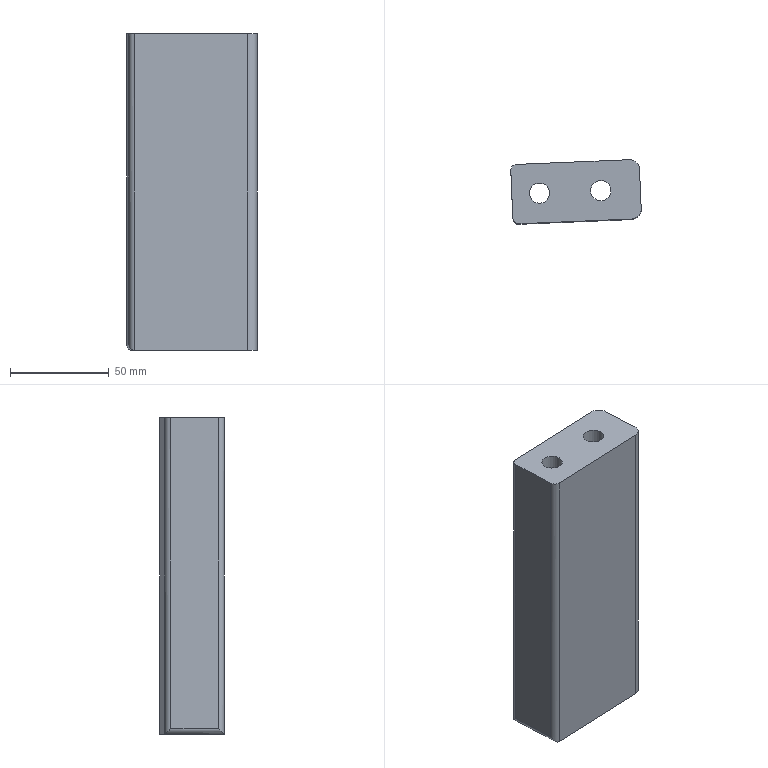Part | NX | features 8 2 | 1 solid | 17 faces | box 65.871 x 32.366 x 160 mm | volume 238451 mm3 | cylinder 9 | plane 8 | commonest cylinder face diameters 6 x3 10 x2 10.3 x2 18 x2
STEP:
#1=CARTESIAN_POINT('',(3750.311,363.335,-69.));
#2=VERTEX_POINT('',#1);
#3=CARTESIAN_POINT('',(3750.311,363.335,91.));
#4=VERTEX_POINT('',#3);
#5=CARTESIAN_POINT('',(3750.311,363.335,-9.));
#6=DIRECTION('',(0.,0.,1.));
#7=VECTOR('',#6,1000.);
#8=LINE('',#5,#7);
#9=EDGE_CURVE('',#2,#4,#8,.T.);
#10=ORIENTED_EDGE('',*,*,#9,.F.);
#11=CARTESIAN_POINT('',(3693.361,360.951,-69.));
#12=VERTEX_POINT('',#11);
#13=CARTESIAN_POINT('',(3740.32,362.917,-69.));
#14=DIRECTION('',(-0.9991,-0.04184,0.));
#15=VECTOR('',#14,1000.);
#16=LINE('',#13,#15);
#17=EDGE_CURVE('',#2,#12,#16,.T.);
#18=ORIENTED_EDGE('',*,*,#17,.T.);
#19=CARTESIAN_POINT('',(3693.361,360.951,91.));
#20=VERTEX_POINT('',#19);
#21=CARTESIAN_POINT('',(3693.361,360.951,-9.));
#22=DIRECTION('',(0.,0.,-1.));
#23=VECTOR('',#22,1000.);
#24=LINE('',#21,#23);
#25=EDGE_CURVE('',#20,#12,#24,.T.);
#26=ORIENTED_EDGE('',*,*,#25,.F.);
#27=CARTESIAN_POINT('',(3740.32,362.917,91.));
#28=DIRECTION('',(-0.9991,-0.04184,0.));
#29=VECTOR('',#28,1000.);
#30=LINE('',#27,#29);
#31=EDGE_CURVE('',#4,#20,#30,.T.);
#32=ORIENTED_EDGE('',*,*,#31,.F.);
#33=EDGE_LOOP('',(#10,#18,#26,#32));
#34=FACE_BOUND('',#33,.T.);
#35=CARTESIAN_POINT('',(3740.32,362.917,-9.));
#36=DIRECTION('',(-0.04184,0.9991,0.));
#37=DIRECTION('',(0.,0.,1.));
#38=AXIS2_PLACEMENT_3D('',#35,#36,#37);
#39=PLANE('',#38);
#40=ADVANCED_FACE('',(#34),#39,.T.);
#41=CARTESIAN_POINT('',(3756.353,338.567,-69.));
#42=VERTEX_POINT('',#41);
#43=CARTESIAN_POINT('',(3756.353,338.567,91.));
#44=VERTEX_POINT('',#43);
#45=CARTESIAN_POINT('',(3756.353,338.567,-9.));
#46=DIRECTION('',(0.,0.,1.));
#47=VECTOR('',#46,1000.);
#48=LINE('',#45,#47);
#49=EDGE_CURVE('',#42,#44,#48,.T.);
#50=ORIENTED_EDGE('',*,*,#49,.F.);
#51=CARTESIAN_POINT('',(3755.516,358.549,-69.));
#52=VERTEX_POINT('',#51);
#53=CARTESIAN_POINT('',(3755.934,348.558,-69.));
#54=DIRECTION('',(-0.04184,0.9991,0.));
#55=VECTOR('',#54,1000.);
#56=LINE('',#53,#55);
#57=EDGE_CURVE('',#42,#52,#56,.T.);
#58=ORIENTED_EDGE('',*,*,#57,.T.);
#59=CARTESIAN_POINT('',(3755.516,358.549,91.));
#60=VERTEX_POINT('',#59);
#61=CARTESIAN_POINT('',(3755.516,358.549,-9.));
#62=DIRECTION('',(0.,0.,-1.));
#63=VECTOR('',#62,1000.);
#64=LINE('',#61,#63);
#65=EDGE_CURVE('',#60,#52,#64,.T.);
#66=ORIENTED_EDGE('',*,*,#65,.F.);
#67=CARTESIAN_POINT('',(3755.934,348.558,91.));
#68=DIRECTION('',(-0.04184,0.9991,0.));
#69=VECTOR('',#68,1000.);
#70=LINE('',#67,#69);
#71=EDGE_CURVE('',#44,#60,#70,.T.);
#72=ORIENTED_EDGE('',*,*,#71,.F.);
#73=EDGE_LOOP('',(#50,#58,#66,#72));
#74=FACE_BOUND('',#73,.T.);
#75=CARTESIAN_POINT('',(3755.934,348.558,-9.));
#76=DIRECTION('',(0.9991,0.04184,0.));
#77=DIRECTION('',(0.,0.,-1.));
#78=AXIS2_PLACEMENT_3D('',#75,#76,#77);
#79=PLANE('',#78);
#80=ADVANCED_FACE('',(#74),#79,.T.);
#81=CARTESIAN_POINT('',(3690.489,357.828,-66.));
#82=VERTEX_POINT('',#81);
#83=CARTESIAN_POINT('',(3690.489,357.828,91.));
#84=VERTEX_POINT('',#83);
#85=CARTESIAN_POINT('',(3690.489,357.828,-9.));
#86=DIRECTION('',(0.,0.,1.));
#87=VECTOR('',#86,1000.);
#88=LINE('',#85,#87);
#89=EDGE_CURVE('',#82,#84,#88,.T.);
#90=ORIENTED_EDGE('',*,*,#89,.F.);
#91=CARTESIAN_POINT('',(3691.493,333.849,-66.));
#92=VERTEX_POINT('',#91);
#93=CARTESIAN_POINT('',(3690.991,345.838,-66.));
#94=DIRECTION('',(0.04184,-0.9991,0.));
#95=VECTOR('',#94,1000.);
#96=LINE('',#93,#95);
#97=EDGE_CURVE('',#82,#92,#96,.T.);
#98=ORIENTED_EDGE('',*,*,#97,.T.);
#99=CARTESIAN_POINT('',(3691.493,333.849,91.));
#100=VERTEX_POINT('',#99);
#101=CARTESIAN_POINT('',(3691.493,333.849,-9.));
#102=DIRECTION('',(0.,0.,-1.));
#103=VECTOR('',#102,1000.);
#104=LINE('',#101,#103);
#105=EDGE_CURVE('',#100,#92,#104,.T.);
#106=ORIENTED_EDGE('',*,*,#105,.F.);
#107=CARTESIAN_POINT('',(3690.991,345.838,91.));
#108=DIRECTION('',(0.04184,-0.9991,0.));
#109=VECTOR('',#108,1000.);
#110=LINE('',#107,#109);
#111=EDGE_CURVE('',#84,#100,#110,.T.);
#112=ORIENTED_EDGE('',*,*,#111,.F.);
#113=EDGE_LOOP('',(#90,#98,#106,#112));
#114=FACE_BOUND('',#113,.T.);
#115=CARTESIAN_POINT('',(3690.991,345.838,-9.));
#116=DIRECTION('',(-0.9991,-0.04184,0.));
#117=DIRECTION('',(0.,0.,1.));
#118=AXIS2_PLACEMENT_3D('',#115,#116,#117);
#119=PLANE('',#118);
#120=ADVANCED_FACE('',(#114),#119,.T.);
#121=ORIENTED_EDGE('',*,*,#25,.T.);
#122=CARTESIAN_POINT('',(3693.487,357.953,-66.));
#123=DIRECTION('',(-0.02958,0.7065,0.7071));
#124=DIRECTION('',(-0.02958,0.7065,-0.7071));
#125=AXIS2_PLACEMENT_3D('',#122,#123,#124);
#126=ELLIPSE('',#125,4.243,3.);
#127=EDGE_CURVE('',#12,#82,#126,.T.);
#128=ORIENTED_EDGE('',*,*,#127,.T.);
#129=ORIENTED_EDGE('',*,*,#89,.T.);
#130=CARTESIAN_POINT('',(3693.487,357.953,91.));
#131=DIRECTION('',(0.,0.,-1.));
#132=DIRECTION('',(1.,0.,0.));
#133=AXIS2_PLACEMENT_3D('',#130,#131,#132);
#134=CIRCLE('',#133,3.);
#135=EDGE_CURVE('',#84,#20,#134,.T.);
#136=ORIENTED_EDGE('',*,*,#135,.T.);
#137=EDGE_LOOP('',(#121,#128,#129,#136));
#138=FACE_BOUND('',#137,.T.);
#139=CARTESIAN_POINT('',(3693.487,357.953,-9.));
#140=DIRECTION('',(0.,0.,-1.));
#141=DIRECTION('',(1.,0.,0.));
#142=AXIS2_PLACEMENT_3D('',#139,#140,#141);
#143=CYLINDRICAL_SURFACE('',#142,3.);
#144=ADVANCED_FACE('',(#138),#143,.T.);
#145=ORIENTED_EDGE('',*,*,#65,.T.);
#146=CARTESIAN_POINT('',(3750.52,358.34,-69.));
#147=DIRECTION('',(0.,0.,1.));
#148=DIRECTION('',(-1.,0.,0.));
#149=AXIS2_PLACEMENT_3D('',#146,#147,#148);
#150=CIRCLE('',#149,5.);
#151=EDGE_CURVE('',#52,#2,#150,.T.);
#152=ORIENTED_EDGE('',*,*,#151,.T.);
#153=ORIENTED_EDGE('',*,*,#9,.T.);
#154=CARTESIAN_POINT('',(3750.52,358.34,91.));
#155=DIRECTION('',(0.,0.,-1.));
#156=DIRECTION('',(-0.9991,-0.04184,0.));
#157=AXIS2_PLACEMENT_3D('',#154,#155,#156);
#158=CIRCLE('',#157,5.);
#159=EDGE_CURVE('',#4,#60,#158,.T.);
#160=ORIENTED_EDGE('',*,*,#159,.T.);
#161=EDGE_LOOP('',(#145,#152,#153,#160));
#162=FACE_BOUND('',#161,.T.);
#163=CARTESIAN_POINT('',(3750.52,358.34,-9.));
#164=DIRECTION('',(0.,0.,1.));
#165=DIRECTION('',(0.9991,0.04184,0.));
#166=AXIS2_PLACEMENT_3D('',#163,#164,#165);
#167=CYLINDRICAL_SURFACE('',#166,5.);
#168=ADVANCED_FACE('',(#162),#167,.T.);
#169=CARTESIAN_POINT('',(3744.952,347.721,61.));
#170=VERTEX_POINT('',#169);
#171=CARTESIAN_POINT('',(3735.952,347.721,61.));
#172=DIRECTION('',(0.,0.,-1.));
#173=DIRECTION('',(1.,0.,0.));
#174=AXIS2_PLACEMENT_3D('',#171,#172,#173);
#175=CIRCLE('',#174,9.);
#176=EDGE_CURVE('',#170,#170,#175,.T.);
#177=ORIENTED_EDGE('',*,*,#176,.F.);
#178=EDGE_LOOP('',(#177));
#179=FACE_BOUND('',#178,.T.);
#180=CARTESIAN_POINT('',(3726.952,347.721,-69.));
#181=VERTEX_POINT('',#180);
#182=CARTESIAN_POINT('',(3735.952,347.721,-69.));
#183=DIRECTION('',(0.,0.,1.));
#184=DIRECTION('',(-1.,0.,0.));
#185=AXIS2_PLACEMENT_3D('',#182,#183,#184);
#186=CIRCLE('',#185,9.);
#187=EDGE_CURVE('',#181,#181,#186,.T.);
#188=ORIENTED_EDGE('',*,*,#187,.F.);
#189=EDGE_LOOP('',(#188));
#190=FACE_BOUND('',#189,.T.);
#191=CARTESIAN_POINT('',(3735.952,347.721,-9.));
#192=DIRECTION('',(0.,0.,1.));
#193=DIRECTION('',(0.9991,0.04184,0.));
#194=AXIS2_PLACEMENT_3D('',#191,#192,#193);
#195=CYLINDRICAL_SURFACE('',#194,9.);
#196=ADVANCED_FACE('',(#179,#190),#195,.F.);
#197=CARTESIAN_POINT('',(3741.102,347.721,91.));
#198=VERTEX_POINT('',#197);
#199=CARTESIAN_POINT('',(3735.952,347.721,91.));
#200=DIRECTION('',(0.,0.,1.));
#201=DIRECTION('',(1.,0.,0.));
#202=AXIS2_PLACEMENT_3D('',#199,#200,#201);
#203=CIRCLE('',#202,5.15);
#204=EDGE_CURVE('',#198,#198,#203,.T.);
#205=ORIENTED_EDGE('',*,*,#204,.F.);
#206=EDGE_LOOP('',(#205));
#207=FACE_BOUND('',#206,.T.);
#208=CARTESIAN_POINT('',(3694.616,330.977,91.));
#209=VERTEX_POINT('',#208);
#210=CARTESIAN_POINT('',(3751.566,333.362,91.));
#211=VERTEX_POINT('',#210);
#212=CARTESIAN_POINT('',(3741.575,332.943,91.));
#213=DIRECTION('',(0.9991,0.04184,0.));
#214=VECTOR('',#213,1000.);
#215=LINE('',#212,#214);
#216=EDGE_CURVE('',#209,#211,#215,.T.);
#217=ORIENTED_EDGE('',*,*,#216,.T.);
#218=CARTESIAN_POINT('',(3751.357,338.357,91.));
#219=DIRECTION('',(0.,0.,-1.));
#220=DIRECTION('',(-0.9991,-0.04184,0.));
#221=AXIS2_PLACEMENT_3D('',#218,#219,#220);
#222=CIRCLE('',#221,5.);
#223=EDGE_CURVE('',#44,#211,#222,.T.);
#224=ORIENTED_EDGE('',*,*,#223,.F.);
#225=ORIENTED_EDGE('',*,*,#71,.T.);
#226=ORIENTED_EDGE('',*,*,#159,.F.);
#227=ORIENTED_EDGE('',*,*,#31,.T.);
#228=ORIENTED_EDGE('',*,*,#135,.F.);
#229=ORIENTED_EDGE('',*,*,#111,.T.);
#230=CARTESIAN_POINT('',(3694.491,333.974,91.));
#231=DIRECTION('',(0.,0.,-1.));
#232=DIRECTION('',(1.,0.,0.));
#233=AXIS2_PLACEMENT_3D('',#230,#231,#232);
#234=CIRCLE('',#233,3.);
#235=EDGE_CURVE('',#209,#100,#234,.T.);
#236=ORIENTED_EDGE('',*,*,#235,.F.);
#237=EDGE_LOOP('',(#217,#224,#225,#226,#227,#228,#229,#236));
#238=FACE_BOUND('',#237,.T.);
#239=CARTESIAN_POINT('',(3710.129,346.424,91.));
#240=VERTEX_POINT('',#239);
#241=CARTESIAN_POINT('',(3704.979,346.424,91.));
#242=DIRECTION('',(0.,0.,1.));
#243=DIRECTION('',(1.,0.,0.));
#244=AXIS2_PLACEMENT_3D('',#241,#242,#243);
#245=CIRCLE('',#244,5.15);
#246=EDGE_CURVE('',#240,#240,#245,.T.);
#247=ORIENTED_EDGE('',*,*,#246,.F.);
#248=EDGE_LOOP('',(#247));
#249=FACE_BOUND('',#248,.T.);
#250=CARTESIAN_POINT('',(3740.948,347.93,91.));
#251=DIRECTION('',(0.,0.,1.));
#252=DIRECTION('',(0.9991,0.04184,0.));
#253=AXIS2_PLACEMENT_3D('',#250,#251,#252);
#254=PLANE('',#253);
#255=ADVANCED_FACE('',(#207,#238,#249),#254,.T.);
#256=CARTESIAN_POINT('',(3694.616,330.977,-69.));
#257=VERTEX_POINT('',#256);
#258=CARTESIAN_POINT('',(3694.616,330.977,-9.));
#259=DIRECTION('',(0.,0.,1.));
#260=VECTOR('',#259,1000.);
#261=LINE('',#258,#260);
#262=EDGE_CURVE('',#257,#209,#261,.T.);
#263=ORIENTED_EDGE('',*,*,#262,.F.);
#264=CARTESIAN_POINT('',(3751.566,333.362,-69.));
#265=VERTEX_POINT('',#264);
#266=CARTESIAN_POINT('',(3741.575,332.943,-69.));
#267=DIRECTION('',(-0.9991,-0.04184,0.));
#268=VECTOR('',#267,1000.);
#269=LINE('',#266,#268);
#270=EDGE_CURVE('',#265,#257,#269,.T.);
#271=ORIENTED_EDGE('',*,*,#270,.F.);
#272=CARTESIAN_POINT('',(3751.566,333.362,-9.));
#273=DIRECTION('',(0.,0.,-1.));
#274=VECTOR('',#273,1000.);
#275=LINE('',#272,#274);
#276=EDGE_CURVE('',#211,#265,#275,.T.);
#277=ORIENTED_EDGE('',*,*,#276,.F.);
#278=ORIENTED_EDGE('',*,*,#216,.F.);
#279=EDGE_LOOP('',(#263,#271,#277,#278));
#280=FACE_BOUND('',#279,.T.);
#281=CARTESIAN_POINT('',(3741.575,332.943,-9.));
#282=DIRECTION('',(0.04184,-0.9991,0.));
#283=DIRECTION('',(0.,0.,-1.));
#284=AXIS2_PLACEMENT_3D('',#281,#282,#283);
#285=PLANE('',#284);
#286=ADVANCED_FACE('',(#280),#285,.T.);
#287=ORIENTED_EDGE('',*,*,#276,.T.);
#288=CARTESIAN_POINT('',(3751.357,338.357,-69.));
#289=DIRECTION('',(0.,0.,-1.));
#290=DIRECTION('',(-1.,0.,0.));
#291=AXIS2_PLACEMENT_3D('',#288,#289,#290);
#292=CIRCLE('',#291,5.);
#293=EDGE_CURVE('',#42,#265,#292,.T.);
#294=ORIENTED_EDGE('',*,*,#293,.F.);
#295=ORIENTED_EDGE('',*,*,#49,.T.);
#296=ORIENTED_EDGE('',*,*,#223,.T.);
#297=EDGE_LOOP('',(#287,#294,#295,#296));
#298=FACE_BOUND('',#297,.T.);
#299=CARTESIAN_POINT('',(3751.357,338.357,-9.));
#300=DIRECTION('',(0.,0.,1.));
#301=DIRECTION('',(0.9991,0.04184,0.));
#302=AXIS2_PLACEMENT_3D('',#299,#300,#301);
#303=CYLINDRICAL_SURFACE('',#302,5.);
#304=ADVANCED_FACE('',(#298),#303,.T.);
#305=ORIENTED_EDGE('',*,*,#105,.T.);
#306=CARTESIAN_POINT('',(3694.491,333.974,-66.));
#307=DIRECTION('',(0.02958,-0.7065,0.7071));
#308=DIRECTION('',(0.02958,-0.7065,-0.7071));
#309=AXIS2_PLACEMENT_3D('',#306,#307,#308);
#310=ELLIPSE('',#309,4.243,3.);
#311=EDGE_CURVE('',#92,#257,#310,.T.);
#312=ORIENTED_EDGE('',*,*,#311,.T.);
#313=ORIENTED_EDGE('',*,*,#262,.T.);
#314=ORIENTED_EDGE('',*,*,#235,.T.);
#315=EDGE_LOOP('',(#305,#312,#313,#314));
#316=FACE_BOUND('',#315,.T.);
#317=CARTESIAN_POINT('',(3694.491,333.974,-9.));
#318=DIRECTION('',(0.,0.,-1.));
#319=DIRECTION('',(1.,0.,0.));
#320=AXIS2_PLACEMENT_3D('',#317,#318,#319);
#321=CYLINDRICAL_SURFACE('',#320,3.);
#322=ADVANCED_FACE('',(#316),#321,.T.);
#323=CARTESIAN_POINT('',(3741.102,347.721,61.));
#324=VERTEX_POINT('',#323);
#325=CARTESIAN_POINT('',(3735.952,347.721,61.));
#326=DIRECTION('',(0.,0.,-1.));
#327=DIRECTION('',(1.,0.,0.));
#328=AXIS2_PLACEMENT_3D('',#325,#326,#327);
#329=CIRCLE('',#328,5.15);
#330=EDGE_CURVE('',#324,#324,#329,.T.);
#331=ORIENTED_EDGE('',*,*,#330,.T.);
#332=EDGE_LOOP('',(#331));
#333=FACE_BOUND('',#332,.T.);
#334=ORIENTED_EDGE('',*,*,#204,.T.);
#335=EDGE_LOOP('',(#334));
#336=FACE_BOUND('',#335,.T.);
#337=CARTESIAN_POINT('',(3735.952,347.721,-9.));
#338=DIRECTION('',(0.,0.,1.));
#339=DIRECTION('',(0.9991,0.04184,0.));
#340=AXIS2_PLACEMENT_3D('',#337,#338,#339);
#341=CYLINDRICAL_SURFACE('',#340,5.15);
#342=ADVANCED_FACE('',(#333,#336),#341,.F.);
#343=ORIENTED_EDGE('',*,*,#330,.F.);
#344=EDGE_LOOP('',(#343));
#345=FACE_BOUND('',#344,.T.);
#346=ORIENTED_EDGE('',*,*,#176,.T.);
#347=EDGE_LOOP('',(#346));
#348=FACE_BOUND('',#347,.T.);
#349=CARTESIAN_POINT('',(3752.499,412.84,61.));
#350=DIRECTION('',(0.,0.,1.));
#351=DIRECTION('',(-1.,0.,0.));
#352=AXIS2_PLACEMENT_3D('',#349,#350,#351);
#353=PLANE('',#352);
#354=ADVANCED_FACE('',(#345,#348),#353,.F.);
#355=CARTESIAN_POINT('',(3710.129,346.424,61.));
#356=VERTEX_POINT('',#355);
#357=CARTESIAN_POINT('',(3704.979,346.424,61.));
#358=DIRECTION('',(0.,0.,-1.));
#359=DIRECTION('',(1.,0.,0.));
#360=AXIS2_PLACEMENT_3D('',#357,#358,#359);
#361=CIRCLE('',#360,5.15);
#362=EDGE_CURVE('',#356,#356,#361,.T.);
#363=ORIENTED_EDGE('',*,*,#362,.T.);
#364=EDGE_LOOP('',(#363));
#365=FACE_BOUND('',#364,.T.);
#366=ORIENTED_EDGE('',*,*,#246,.T.);
#367=EDGE_LOOP('',(#366));
#368=FACE_BOUND('',#367,.T.);
#369=CARTESIAN_POINT('',(3704.979,346.424,-9.));
#370=DIRECTION('',(0.,0.,1.));
#371=DIRECTION('',(0.9991,0.04184,0.));
#372=AXIS2_PLACEMENT_3D('',#369,#370,#371);
#373=CYLINDRICAL_SURFACE('',#372,5.15);
#374=ADVANCED_FACE('',(#365,#368),#373,.F.);
#375=ORIENTED_EDGE('',*,*,#362,.F.);
#376=EDGE_LOOP('',(#375));
#377=FACE_BOUND('',#376,.T.);
#378=CARTESIAN_POINT('',(3713.979,346.424,61.));
#379=VERTEX_POINT('',#378);
#380=CARTESIAN_POINT('',(3704.979,346.424,61.));
#381=DIRECTION('',(0.,0.,-1.));
#382=DIRECTION('',(1.,0.,0.));
#383=AXIS2_PLACEMENT_3D('',#380,#381,#382);
#384=CIRCLE('',#383,9.);
#385=EDGE_CURVE('',#379,#379,#384,.T.);
#386=ORIENTED_EDGE('',*,*,#385,.T.);
#387=EDGE_LOOP('',(#386));
#388=FACE_BOUND('',#387,.T.);
#389=CARTESIAN_POINT('',(3752.499,412.84,61.));
#390=DIRECTION('',(0.,0.,1.));
#391=DIRECTION('',(-1.,0.,0.));
#392=AXIS2_PLACEMENT_3D('',#389,#390,#391);
#393=PLANE('',#392);
#394=ADVANCED_FACE('',(#377,#388),#393,.F.);
#395=ORIENTED_EDGE('',*,*,#385,.F.);
#396=EDGE_LOOP('',(#395));
#397=FACE_BOUND('',#396,.T.);
#398=CARTESIAN_POINT('',(3695.979,346.424,-69.));
#399=VERTEX_POINT('',#398);
#400=CARTESIAN_POINT('',(3704.979,346.424,-69.));
#401=DIRECTION('',(0.,0.,-1.));
#402=DIRECTION('',(-1.,0.,0.));
#403=AXIS2_PLACEMENT_3D('',#400,#401,#402);
#404=CIRCLE('',#403,9.);
#405=EDGE_CURVE('',#399,#399,#404,.T.);
#406=ORIENTED_EDGE('',*,*,#405,.T.);
#407=EDGE_LOOP('',(#406));
#408=FACE_BOUND('',#407,.T.);
#409=CARTESIAN_POINT('',(3704.979,346.424,-9.));
#410=DIRECTION('',(0.,0.,1.));
#411=DIRECTION('',(0.9991,0.04184,0.));
#412=AXIS2_PLACEMENT_3D('',#409,#410,#411);
#413=CYLINDRICAL_SURFACE('',#412,9.);
#414=ADVANCED_FACE('',(#397,#408),#413,.F.);
#415=ORIENTED_EDGE('',*,*,#405,.F.);
#416=EDGE_LOOP('',(#415));
#417=FACE_BOUND('',#416,.T.);
#418=ORIENTED_EDGE('',*,*,#270,.T.);
#419=CARTESIAN_POINT('',(3693.99,345.925,-69.));
#420=DIRECTION('',(-0.04184,0.9991,0.));
#421=VECTOR('',#420,1000.);
#422=LINE('',#419,#421);
#423=EDGE_CURVE('',#257,#12,#422,.T.);
#424=ORIENTED_EDGE('',*,*,#423,.T.);
#425=ORIENTED_EDGE('',*,*,#17,.F.);
#426=ORIENTED_EDGE('',*,*,#151,.F.);
#427=ORIENTED_EDGE('',*,*,#57,.F.);
#428=ORIENTED_EDGE('',*,*,#293,.T.);
#429=EDGE_LOOP('',(#418,#424,#425,#426,#427,#428));
#430=FACE_BOUND('',#429,.T.);
#431=ORIENTED_EDGE('',*,*,#187,.T.);
#432=EDGE_LOOP('',(#431));
#433=FACE_BOUND('',#432,.T.);
#434=CARTESIAN_POINT('',(3723.422,347.157,-69.));
#435=DIRECTION('',(0.,0.,-1.));
#436=DIRECTION('',(1.,0.,0.));
#437=AXIS2_PLACEMENT_3D('',#434,#435,#436);
#438=PLANE('',#437);
#439=ADVANCED_FACE('',(#417,#430,#433),#438,.T.);
#440=ORIENTED_EDGE('',*,*,#127,.F.);
#441=ORIENTED_EDGE('',*,*,#423,.F.);
#442=ORIENTED_EDGE('',*,*,#311,.F.);
#443=ORIENTED_EDGE('',*,*,#97,.F.);
#444=EDGE_LOOP('',(#440,#441,#442,#443));
#445=FACE_BOUND('',#444,.T.);
#446=CARTESIAN_POINT('',(3693.989,345.964,-66.));
#447=DIRECTION('',(0.04184,-0.9991,0.));
#448=DIRECTION('',(-0.9991,-0.04184,0.));
#449=AXIS2_PLACEMENT_3D('',#446,#447,#448);
#450=CYLINDRICAL_SURFACE('',#449,3.);
#451=ADVANCED_FACE('',(#445),#450,.T.);
#452=CLOSED_SHELL('',(#40,#80,#120,#144,#168,#196,#255,#286,#304,#322,#342,#354,#374,#394,#414,#439,#451));
#453=MANIFOLD_SOLID_BREP('',#452);
#454=(LENGTH_UNIT()NAMED_UNIT(*)SI_UNIT(.MILLI.,.METRE.));
#455=UNCERTAINTY_MEASURE_WITH_UNIT(LENGTH_MEASURE(0.00001),#454,'','');
#456=(NAMED_UNIT(*)PLANE_ANGLE_UNIT()SI_UNIT($,.RADIAN.));
#457=(NAMED_UNIT(*)SI_UNIT($,.STERADIAN.)SOLID_ANGLE_UNIT());
#458=(GEOMETRIC_REPRESENTATION_CONTEXT(3)GLOBAL_UNCERTAINTY_ASSIGNED_CONTEXT((#455))GLOBAL_UNIT_ASSIGNED_CONTEXT((#454,#456,#457))REPRESENTATION_CONTEXT('',''));
#459=ADVANCED_BREP_SHAPE_REPRESENTATION('',(#453),#458);